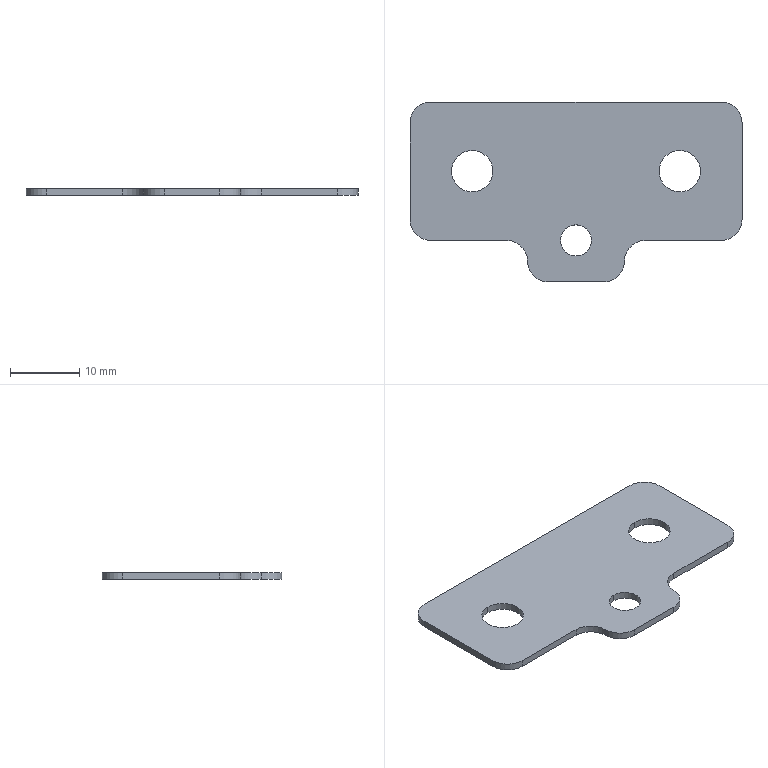Part | STEP file | J454-EBZ05-37-04-Part-1-1 | 1 solid | 22 faces | box 48 x 26 x 1 mm | volume 963.821 mm3 | cylinder 14 | plane 8 | commonest cylinder face diameters 6 x12 4.5 x2
STEP:
#1=CARTESIAN_POINT('',(24.,1.75,1.));
#2=VERTEX_POINT('',#1);
#3=CARTESIAN_POINT('',(24.,6.25,1.));
#4=VERTEX_POINT('',#3);
#5=CARTESIAN_POINT('',(24.,4.,1.));
#6=DIRECTION('',(0.,0.,-1.));
#7=DIRECTION('',(0.,1.,0.));
#8=AXIS2_PLACEMENT_3D('',#5,#6,#7);
#9=CIRCLE('',#8,2.25);
#10=EDGE_CURVE('',#2,#4,#9,.T.);
#11=ORIENTED_EDGE('',*,*,#10,.F.);
#12=CARTESIAN_POINT('',(24.,1.75,0.));
#13=VERTEX_POINT('',#12);
#14=CARTESIAN_POINT('',(24.,1.75,1.));
#15=DIRECTION('',(0.,0.,-1.));
#16=VECTOR('',#15,1000.);
#17=LINE('',#14,#16);
#18=EDGE_CURVE('',#2,#13,#17,.T.);
#19=ORIENTED_EDGE('',*,*,#18,.T.);
#20=CARTESIAN_POINT('',(24.,6.25,0.));
#21=VERTEX_POINT('',#20);
#22=CARTESIAN_POINT('',(24.,4.,0.));
#23=DIRECTION('',(0.,0.,1.));
#24=DIRECTION('',(0.,-1.,0.));
#25=AXIS2_PLACEMENT_3D('',#22,#23,#24);
#26=CIRCLE('',#25,2.25);
#27=EDGE_CURVE('',#21,#13,#26,.T.);
#28=ORIENTED_EDGE('',*,*,#27,.F.);
#29=CARTESIAN_POINT('',(24.,6.25,1.));
#30=DIRECTION('',(0.,0.,-1.));
#31=VECTOR('',#30,1000.);
#32=LINE('',#29,#31);
#33=EDGE_CURVE('',#4,#21,#32,.T.);
#34=ORIENTED_EDGE('',*,*,#33,.F.);
#35=EDGE_LOOP('',(#11,#19,#28,#34));
#36=FACE_OUTER_BOUND('',#35,.T.);
#37=CARTESIAN_POINT('',(24.,4.,1.));
#38=DIRECTION('',(0.,0.,-1.));
#39=DIRECTION('',(0.,1.,0.));
#40=AXIS2_PLACEMENT_3D('',#37,#38,#39);
#41=CYLINDRICAL_SURFACE('',#40,2.25);
#42=ADVANCED_FACE('',(#36),#41,.F.);
#43=CARTESIAN_POINT('',(9.,17.,0.));
#44=VERTEX_POINT('',#43);
#45=CARTESIAN_POINT('',(9.,11.,0.));
#46=VERTEX_POINT('',#45);
#47=CARTESIAN_POINT('',(9.,14.,0.));
#48=DIRECTION('',(0.,0.,1.));
#49=DIRECTION('',(0.,-1.,0.));
#50=AXIS2_PLACEMENT_3D('',#47,#48,#49);
#51=CIRCLE('',#50,3.);
#52=EDGE_CURVE('',#44,#46,#51,.T.);
#53=ORIENTED_EDGE('',*,*,#52,.F.);
#54=CARTESIAN_POINT('',(9.,17.,1.));
#55=VERTEX_POINT('',#54);
#56=CARTESIAN_POINT('',(9.,17.,0.));
#57=DIRECTION('',(0.,0.,1.));
#58=VECTOR('',#57,1000.);
#59=LINE('',#56,#58);
#60=EDGE_CURVE('',#44,#55,#59,.T.);
#61=ORIENTED_EDGE('',*,*,#60,.T.);
#62=CARTESIAN_POINT('',(9.,11.,1.));
#63=VERTEX_POINT('',#62);
#64=CARTESIAN_POINT('',(9.,14.,1.));
#65=DIRECTION('',(0.,0.,-1.));
#66=DIRECTION('',(0.,1.,0.));
#67=AXIS2_PLACEMENT_3D('',#64,#65,#66);
#68=CIRCLE('',#67,3.);
#69=EDGE_CURVE('',#63,#55,#68,.T.);
#70=ORIENTED_EDGE('',*,*,#69,.F.);
#71=CARTESIAN_POINT('',(9.,11.,0.));
#72=DIRECTION('',(0.,0.,1.));
#73=VECTOR('',#72,1000.);
#74=LINE('',#71,#73);
#75=EDGE_CURVE('',#46,#63,#74,.T.);
#76=ORIENTED_EDGE('',*,*,#75,.F.);
#77=EDGE_LOOP('',(#53,#61,#70,#76));
#78=FACE_OUTER_BOUND('',#77,.T.);
#79=CARTESIAN_POINT('',(9.,14.,0.));
#80=DIRECTION('',(0.,0.,1.));
#81=DIRECTION('',(0.,-1.,0.));
#82=AXIS2_PLACEMENT_3D('',#79,#80,#81);
#83=CYLINDRICAL_SURFACE('',#82,3.);
#84=ADVANCED_FACE('',(#78),#83,.F.);
#85=CARTESIAN_POINT('',(39.,17.,0.));
#86=VERTEX_POINT('',#85);
#87=CARTESIAN_POINT('',(39.,11.,0.));
#88=VERTEX_POINT('',#87);
#89=CARTESIAN_POINT('',(39.,14.,0.));
#90=DIRECTION('',(0.,0.,1.));
#91=DIRECTION('',(0.,-1.,0.));
#92=AXIS2_PLACEMENT_3D('',#89,#90,#91);
#93=CIRCLE('',#92,3.);
#94=EDGE_CURVE('',#86,#88,#93,.T.);
#95=ORIENTED_EDGE('',*,*,#94,.F.);
#96=CARTESIAN_POINT('',(39.,17.,1.));
#97=VERTEX_POINT('',#96);
#98=CARTESIAN_POINT('',(39.,17.,0.));
#99=DIRECTION('',(0.,0.,1.));
#100=VECTOR('',#99,1000.);
#101=LINE('',#98,#100);
#102=EDGE_CURVE('',#86,#97,#101,.T.);
#103=ORIENTED_EDGE('',*,*,#102,.T.);
#104=CARTESIAN_POINT('',(39.,11.,1.));
#105=VERTEX_POINT('',#104);
#106=CARTESIAN_POINT('',(39.,14.,1.));
#107=DIRECTION('',(0.,0.,-1.));
#108=DIRECTION('',(0.,1.,0.));
#109=AXIS2_PLACEMENT_3D('',#106,#107,#108);
#110=CIRCLE('',#109,3.);
#111=EDGE_CURVE('',#105,#97,#110,.T.);
#112=ORIENTED_EDGE('',*,*,#111,.F.);
#113=CARTESIAN_POINT('',(39.,11.,0.));
#114=DIRECTION('',(0.,0.,1.));
#115=VECTOR('',#114,1000.);
#116=LINE('',#113,#115);
#117=EDGE_CURVE('',#88,#105,#116,.T.);
#118=ORIENTED_EDGE('',*,*,#117,.F.);
#119=EDGE_LOOP('',(#95,#103,#112,#118));
#120=FACE_OUTER_BOUND('',#119,.T.);
#121=CARTESIAN_POINT('',(39.,14.,0.));
#122=DIRECTION('',(0.,0.,1.));
#123=DIRECTION('',(0.,-1.,0.));
#124=AXIS2_PLACEMENT_3D('',#121,#122,#123);
#125=CYLINDRICAL_SURFACE('',#124,3.);
#126=ADVANCED_FACE('',(#120),#125,.F.);
#127=CARTESIAN_POINT('',(14.,4.,0.));
#128=VERTEX_POINT('',#127);
#129=CARTESIAN_POINT('',(3.,4.,0.));
#130=VERTEX_POINT('',#129);
#131=CARTESIAN_POINT('',(24.,4.,0.));
#132=DIRECTION('',(-1.,0.,0.));
#133=VECTOR('',#132,1000.);
#134=LINE('',#131,#133);
#135=EDGE_CURVE('',#128,#130,#134,.T.);
#136=ORIENTED_EDGE('',*,*,#135,.F.);
#137=CARTESIAN_POINT('',(14.,4.,1.));
#138=VERTEX_POINT('',#137);
#139=CARTESIAN_POINT('',(14.,4.,1.));
#140=DIRECTION('',(0.,0.,1.));
#141=VECTOR('',#140,1000.);
#142=LINE('',#139,#141);
#143=EDGE_CURVE('',#128,#138,#142,.T.);
#144=ORIENTED_EDGE('',*,*,#143,.T.);
#145=CARTESIAN_POINT('',(3.,4.,1.));
#146=VERTEX_POINT('',#145);
#147=CARTESIAN_POINT('',(24.,4.,1.));
#148=DIRECTION('',(1.,0.,0.));
#149=VECTOR('',#148,1000.);
#150=LINE('',#147,#149);
#151=EDGE_CURVE('',#146,#138,#150,.T.);
#152=ORIENTED_EDGE('',*,*,#151,.F.);
#153=CARTESIAN_POINT('',(3.,4.,0.5));
#154=DIRECTION('',(0.,0.,-1.));
#155=VECTOR('',#154,1000.);
#156=LINE('',#153,#155);
#157=EDGE_CURVE('',#146,#130,#156,.T.);
#158=ORIENTED_EDGE('',*,*,#157,.T.);
#159=EDGE_LOOP('',(#136,#144,#152,#158));
#160=FACE_OUTER_BOUND('',#159,.T.);
#161=CARTESIAN_POINT('',(24.,4.,0.5));
#162=DIRECTION('',(0.,-1.,0.));
#163=DIRECTION('',(0.,0.,-1.));
#164=AXIS2_PLACEMENT_3D('',#161,#162,#163);
#165=PLANE('',#164);
#166=ADVANCED_FACE('',(#160),#165,.T.);
#167=CARTESIAN_POINT('',(45.,24.,1.));
#168=VERTEX_POINT('',#167);
#169=CARTESIAN_POINT('',(3.,24.,1.));
#170=VERTEX_POINT('',#169);
#171=CARTESIAN_POINT('',(24.,24.,1.));
#172=DIRECTION('',(-1.,0.,0.));
#173=VECTOR('',#172,1000.);
#174=LINE('',#171,#173);
#175=EDGE_CURVE('',#168,#170,#174,.T.);
#176=ORIENTED_EDGE('',*,*,#175,.F.);
#177=CARTESIAN_POINT('',(45.,24.,0.));
#178=VERTEX_POINT('',#177);
#179=CARTESIAN_POINT('',(45.,24.,0.5));
#180=DIRECTION('',(0.,0.,-1.));
#181=VECTOR('',#180,1000.);
#182=LINE('',#179,#181);
#183=EDGE_CURVE('',#168,#178,#182,.T.);
#184=ORIENTED_EDGE('',*,*,#183,.T.);
#185=CARTESIAN_POINT('',(3.,24.,0.));
#186=VERTEX_POINT('',#185);
#187=CARTESIAN_POINT('',(24.,24.,0.));
#188=DIRECTION('',(1.,0.,0.));
#189=VECTOR('',#188,1000.);
#190=LINE('',#187,#189);
#191=EDGE_CURVE('',#186,#178,#190,.T.);
#192=ORIENTED_EDGE('',*,*,#191,.F.);
#193=CARTESIAN_POINT('',(3.,24.,0.5));
#194=DIRECTION('',(0.,0.,1.));
#195=VECTOR('',#194,1000.);
#196=LINE('',#193,#195);
#197=EDGE_CURVE('',#186,#170,#196,.T.);
#198=ORIENTED_EDGE('',*,*,#197,.T.);
#199=EDGE_LOOP('',(#176,#184,#192,#198));
#200=FACE_OUTER_BOUND('',#199,.T.);
#201=CARTESIAN_POINT('',(24.,24.,0.5));
#202=DIRECTION('',(0.,1.,0.));
#203=DIRECTION('',(0.,0.,1.));
#204=AXIS2_PLACEMENT_3D('',#201,#202,#203);
#205=PLANE('',#204);
#206=ADVANCED_FACE('',(#200),#205,.T.);
#207=CARTESIAN_POINT('',(0.,7.,0.));
#208=VERTEX_POINT('',#207);
#209=CARTESIAN_POINT('',(0.,21.,0.));
#210=VERTEX_POINT('',#209);
#211=CARTESIAN_POINT('',(0.,4.,0.));
#212=DIRECTION('',(0.,1.,0.));
#213=VECTOR('',#212,1000.);
#214=LINE('',#211,#213);
#215=EDGE_CURVE('',#208,#210,#214,.T.);
#216=ORIENTED_EDGE('',*,*,#215,.F.);
#217=CARTESIAN_POINT('',(0.,7.,1.));
#218=VERTEX_POINT('',#217);
#219=CARTESIAN_POINT('',(0.,7.,0.5));
#220=DIRECTION('',(0.,0.,1.));
#221=VECTOR('',#220,1000.);
#222=LINE('',#219,#221);
#223=EDGE_CURVE('',#208,#218,#222,.T.);
#224=ORIENTED_EDGE('',*,*,#223,.T.);
#225=CARTESIAN_POINT('',(0.,21.,1.));
#226=VERTEX_POINT('',#225);
#227=CARTESIAN_POINT('',(0.,4.,1.));
#228=DIRECTION('',(0.,1.,0.));
#229=VECTOR('',#228,1000.);
#230=LINE('',#227,#229);
#231=EDGE_CURVE('',#218,#226,#230,.T.);
#232=ORIENTED_EDGE('',*,*,#231,.T.);
#233=CARTESIAN_POINT('',(0.,21.,0.5));
#234=DIRECTION('',(0.,0.,-1.));
#235=VECTOR('',#234,1000.);
#236=LINE('',#233,#235);
#237=EDGE_CURVE('',#226,#210,#236,.T.);
#238=ORIENTED_EDGE('',*,*,#237,.T.);
#239=EDGE_LOOP('',(#216,#224,#232,#238));
#240=FACE_OUTER_BOUND('',#239,.T.);
#241=CARTESIAN_POINT('',(0.,4.,0.5));
#242=DIRECTION('',(-1.,0.,0.));
#243=DIRECTION('',(0.,-1.,0.));
#244=AXIS2_PLACEMENT_3D('',#241,#242,#243);
#245=PLANE('',#244);
#246=ADVANCED_FACE('',(#240),#245,.T.);
#247=ORIENTED_EDGE('',*,*,#27,.T.);
#248=CARTESIAN_POINT('',(24.,4.,0.));
#249=DIRECTION('',(0.,0.,1.));
#250=DIRECTION('',(0.,-1.,0.));
#251=AXIS2_PLACEMENT_3D('',#248,#249,#250);
#252=CIRCLE('',#251,2.25);
#253=EDGE_CURVE('',#13,#21,#252,.T.);
#254=ORIENTED_EDGE('',*,*,#253,.T.);
#255=EDGE_LOOP('',(#247,#254));
#256=FACE_BOUND('',#255,.T.);
#257=CARTESIAN_POINT('',(9.,14.,0.));
#258=DIRECTION('',(0.,0.,1.));
#259=DIRECTION('',(0.,-1.,0.));
#260=AXIS2_PLACEMENT_3D('',#257,#258,#259);
#261=CIRCLE('',#260,3.);
#262=EDGE_CURVE('',#46,#44,#261,.T.);
#263=ORIENTED_EDGE('',*,*,#262,.T.);
#264=ORIENTED_EDGE('',*,*,#52,.T.);
#265=EDGE_LOOP('',(#263,#264));
#266=FACE_BOUND('',#265,.T.);
#267=CARTESIAN_POINT('',(39.,14.,0.));
#268=DIRECTION('',(0.,0.,1.));
#269=DIRECTION('',(0.,-1.,0.));
#270=AXIS2_PLACEMENT_3D('',#267,#268,#269);
#271=CIRCLE('',#270,3.);
#272=EDGE_CURVE('',#88,#86,#271,.T.);
#273=ORIENTED_EDGE('',*,*,#272,.T.);
#274=ORIENTED_EDGE('',*,*,#94,.T.);
#275=EDGE_LOOP('',(#273,#274));
#276=FACE_BOUND('',#275,.T.);
#277=CARTESIAN_POINT('',(28.,-2.,0.));
#278=VERTEX_POINT('',#277);
#279=CARTESIAN_POINT('',(20.,-2.,0.));
#280=VERTEX_POINT('',#279);
#281=CARTESIAN_POINT('',(24.,-2.,0.));
#282=DIRECTION('',(-1.,0.,0.));
#283=VECTOR('',#282,1000.);
#284=LINE('',#281,#283);
#285=EDGE_CURVE('',#278,#280,#284,.T.);
#286=ORIENTED_EDGE('',*,*,#285,.T.);
#287=CARTESIAN_POINT('',(17.,1.,0.));
#288=VERTEX_POINT('',#287);
#289=CARTESIAN_POINT('',(20.,1.,0.));
#290=DIRECTION('',(0.,0.,-1.));
#291=DIRECTION('',(0.,1.,0.));
#292=AXIS2_PLACEMENT_3D('',#289,#290,#291);
#293=CIRCLE('',#292,3.);
#294=EDGE_CURVE('',#280,#288,#293,.T.);
#295=ORIENTED_EDGE('',*,*,#294,.T.);
#296=CARTESIAN_POINT('',(14.,1.,0.));
#297=DIRECTION('',(0.,0.,1.));
#298=DIRECTION('',(0.,1.,0.));
#299=AXIS2_PLACEMENT_3D('',#296,#297,#298);
#300=CIRCLE('',#299,3.);
#301=EDGE_CURVE('',#288,#128,#300,.T.);
#302=ORIENTED_EDGE('',*,*,#301,.T.);
#303=ORIENTED_EDGE('',*,*,#135,.T.);
#304=CARTESIAN_POINT('',(3.,7.,0.));
#305=DIRECTION('',(0.,0.,-1.));
#306=DIRECTION('',(0.,1.,0.));
#307=AXIS2_PLACEMENT_3D('',#304,#305,#306);
#308=CIRCLE('',#307,3.);
#309=EDGE_CURVE('',#130,#208,#308,.T.);
#310=ORIENTED_EDGE('',*,*,#309,.T.);
#311=ORIENTED_EDGE('',*,*,#215,.T.);
#312=CARTESIAN_POINT('',(3.,21.,0.));
#313=DIRECTION('',(0.,0.,-1.));
#314=DIRECTION('',(0.,1.,0.));
#315=AXIS2_PLACEMENT_3D('',#312,#313,#314);
#316=CIRCLE('',#315,3.);
#317=EDGE_CURVE('',#210,#186,#316,.T.);
#318=ORIENTED_EDGE('',*,*,#317,.T.);
#319=ORIENTED_EDGE('',*,*,#191,.T.);
#320=CARTESIAN_POINT('',(48.,21.,0.));
#321=VERTEX_POINT('',#320);
#322=CARTESIAN_POINT('',(45.,21.,0.));
#323=DIRECTION('',(0.,0.,-1.));
#324=DIRECTION('',(0.,1.,0.));
#325=AXIS2_PLACEMENT_3D('',#322,#323,#324);
#326=CIRCLE('',#325,3.);
#327=EDGE_CURVE('',#178,#321,#326,.T.);
#328=ORIENTED_EDGE('',*,*,#327,.T.);
#329=CARTESIAN_POINT('',(48.,7.,0.));
#330=VERTEX_POINT('',#329);
#331=CARTESIAN_POINT('',(48.,4.,0.));
#332=DIRECTION('',(0.,1.,0.));
#333=VECTOR('',#332,1000.);
#334=LINE('',#331,#333);
#335=EDGE_CURVE('',#330,#321,#334,.T.);
#336=ORIENTED_EDGE('',*,*,#335,.F.);
#337=CARTESIAN_POINT('',(45.,4.,0.));
#338=VERTEX_POINT('',#337);
#339=CARTESIAN_POINT('',(45.,7.,0.));
#340=DIRECTION('',(0.,0.,-1.));
#341=DIRECTION('',(0.,1.,0.));
#342=AXIS2_PLACEMENT_3D('',#339,#340,#341);
#343=CIRCLE('',#342,3.);
#344=EDGE_CURVE('',#330,#338,#343,.T.);
#345=ORIENTED_EDGE('',*,*,#344,.T.);
#346=CARTESIAN_POINT('',(34.,4.,0.));
#347=VERTEX_POINT('',#346);
#348=CARTESIAN_POINT('',(24.,4.,0.));
#349=DIRECTION('',(-1.,0.,0.));
#350=VECTOR('',#349,1000.);
#351=LINE('',#348,#350);
#352=EDGE_CURVE('',#338,#347,#351,.T.);
#353=ORIENTED_EDGE('',*,*,#352,.T.);
#354=CARTESIAN_POINT('',(31.,1.,0.));
#355=VERTEX_POINT('',#354);
#356=CARTESIAN_POINT('',(34.,1.,0.));
#357=DIRECTION('',(0.,0.,1.));
#358=DIRECTION('',(0.,1.,0.));
#359=AXIS2_PLACEMENT_3D('',#356,#357,#358);
#360=CIRCLE('',#359,3.);
#361=EDGE_CURVE('',#347,#355,#360,.T.);
#362=ORIENTED_EDGE('',*,*,#361,.T.);
#363=CARTESIAN_POINT('',(28.,1.,0.));
#364=DIRECTION('',(0.,0.,-1.));
#365=DIRECTION('',(0.,1.,0.));
#366=AXIS2_PLACEMENT_3D('',#363,#364,#365);
#367=CIRCLE('',#366,3.);
#368=EDGE_CURVE('',#355,#278,#367,.T.);
#369=ORIENTED_EDGE('',*,*,#368,.T.);
#370=EDGE_LOOP('',(#286,#295,#302,#303,#310,#311,#318,#319,#328,#336,#345,#353,#362,#369));
#371=FACE_OUTER_BOUND('',#370,.T.);
#372=CARTESIAN_POINT('',(24.,4.,0.));
#373=DIRECTION('',(0.,0.,-1.));
#374=DIRECTION('',(0.,1.,0.));
#375=AXIS2_PLACEMENT_3D('',#372,#373,#374);
#376=PLANE('',#375);
#377=ADVANCED_FACE('',(#256,#266,#276,#371),#376,.T.);
#378=CARTESIAN_POINT('',(48.,7.,1.));
#379=VERTEX_POINT('',#378);
#380=CARTESIAN_POINT('',(48.,21.,1.));
#381=VERTEX_POINT('',#380);
#382=CARTESIAN_POINT('',(48.,4.,1.));
#383=DIRECTION('',(0.,1.,0.));
#384=VECTOR('',#383,1000.);
#385=LINE('',#382,#384);
#386=EDGE_CURVE('',#379,#381,#385,.T.);
#387=ORIENTED_EDGE('',*,*,#386,.F.);
#388=CARTESIAN_POINT('',(48.,7.,0.5));
#389=DIRECTION('',(0.,0.,-1.));
#390=VECTOR('',#389,1000.);
#391=LINE('',#388,#390);
#392=EDGE_CURVE('',#379,#330,#391,.T.);
#393=ORIENTED_EDGE('',*,*,#392,.T.);
#394=ORIENTED_EDGE('',*,*,#335,.T.);
#395=CARTESIAN_POINT('',(48.,21.,0.5));
#396=DIRECTION('',(0.,0.,1.));
#397=VECTOR('',#396,1000.);
#398=LINE('',#395,#397);
#399=EDGE_CURVE('',#321,#381,#398,.T.);
#400=ORIENTED_EDGE('',*,*,#399,.T.);
#401=EDGE_LOOP('',(#387,#393,#394,#400));
#402=FACE_OUTER_BOUND('',#401,.T.);
#403=CARTESIAN_POINT('',(48.,4.,0.5));
#404=DIRECTION('',(1.,0.,0.));
#405=DIRECTION('',(0.,1.,0.));
#406=AXIS2_PLACEMENT_3D('',#403,#404,#405);
#407=PLANE('',#406);
#408=ADVANCED_FACE('',(#402),#407,.T.);
#409=CARTESIAN_POINT('',(34.,4.,1.));
#410=VERTEX_POINT('',#409);
#411=CARTESIAN_POINT('',(45.,4.,1.));
#412=VERTEX_POINT('',#411);
#413=CARTESIAN_POINT('',(24.,4.,1.));
#414=DIRECTION('',(1.,0.,0.));
#415=VECTOR('',#414,1000.);
#416=LINE('',#413,#415);
#417=EDGE_CURVE('',#410,#412,#416,.T.);
#418=ORIENTED_EDGE('',*,*,#417,.F.);
#419=CARTESIAN_POINT('',(34.,4.,0.));
#420=DIRECTION('',(0.,0.,-1.));
#421=VECTOR('',#420,1000.);
#422=LINE('',#419,#421);
#423=EDGE_CURVE('',#410,#347,#422,.T.);
#424=ORIENTED_EDGE('',*,*,#423,.T.);
#425=ORIENTED_EDGE('',*,*,#352,.F.);
#426=CARTESIAN_POINT('',(45.,4.,0.5));
#427=DIRECTION('',(0.,0.,1.));
#428=VECTOR('',#427,1000.);
#429=LINE('',#426,#428);
#430=EDGE_CURVE('',#338,#412,#429,.T.);
#431=ORIENTED_EDGE('',*,*,#430,.T.);
#432=EDGE_LOOP('',(#418,#424,#425,#431));
#433=FACE_OUTER_BOUND('',#432,.T.);
#434=CARTESIAN_POINT('',(24.,4.,0.5));
#435=DIRECTION('',(0.,-1.,0.));
#436=DIRECTION('',(0.,0.,-1.));
#437=AXIS2_PLACEMENT_3D('',#434,#435,#436);
#438=PLANE('',#437);
#439=ADVANCED_FACE('',(#433),#438,.T.);
#440=CARTESIAN_POINT('',(24.,4.,1.));
#441=DIRECTION('',(0.,0.,-1.));
#442=DIRECTION('',(0.,1.,0.));
#443=AXIS2_PLACEMENT_3D('',#440,#441,#442);
#444=CIRCLE('',#443,2.25);
#445=EDGE_CURVE('',#4,#2,#444,.T.);
#446=ORIENTED_EDGE('',*,*,#445,.T.);
#447=ORIENTED_EDGE('',*,*,#10,.T.);
#448=EDGE_LOOP('',(#446,#447));
#449=FACE_BOUND('',#448,.T.);
#450=ORIENTED_EDGE('',*,*,#69,.T.);
#451=CARTESIAN_POINT('',(9.,14.,1.));
#452=DIRECTION('',(0.,0.,-1.));
#453=DIRECTION('',(0.,1.,0.));
#454=AXIS2_PLACEMENT_3D('',#451,#452,#453);
#455=CIRCLE('',#454,3.);
#456=EDGE_CURVE('',#55,#63,#455,.T.);
#457=ORIENTED_EDGE('',*,*,#456,.T.);
#458=EDGE_LOOP('',(#450,#457));
#459=FACE_BOUND('',#458,.T.);
#460=ORIENTED_EDGE('',*,*,#111,.T.);
#461=CARTESIAN_POINT('',(39.,14.,1.));
#462=DIRECTION('',(0.,0.,-1.));
#463=DIRECTION('',(0.,1.,0.));
#464=AXIS2_PLACEMENT_3D('',#461,#462,#463);
#465=CIRCLE('',#464,3.);
#466=EDGE_CURVE('',#97,#105,#465,.T.);
#467=ORIENTED_EDGE('',*,*,#466,.T.);
#468=EDGE_LOOP('',(#460,#467));
#469=FACE_BOUND('',#468,.T.);
#470=ORIENTED_EDGE('',*,*,#151,.T.);
#471=CARTESIAN_POINT('',(17.,1.,1.));
#472=VERTEX_POINT('',#471);
#473=CARTESIAN_POINT('',(14.,1.,1.));
#474=DIRECTION('',(0.,0.,-1.));
#475=DIRECTION('',(0.,-1.,0.));
#476=AXIS2_PLACEMENT_3D('',#473,#474,#475);
#477=CIRCLE('',#476,3.);
#478=EDGE_CURVE('',#138,#472,#477,.T.);
#479=ORIENTED_EDGE('',*,*,#478,.T.);
#480=CARTESIAN_POINT('',(20.,-2.,1.));
#481=VERTEX_POINT('',#480);
#482=CARTESIAN_POINT('',(20.,1.,1.));
#483=DIRECTION('',(0.,0.,1.));
#484=DIRECTION('',(0.,-1.,0.));
#485=AXIS2_PLACEMENT_3D('',#482,#483,#484);
#486=CIRCLE('',#485,3.);
#487=EDGE_CURVE('',#472,#481,#486,.T.);
#488=ORIENTED_EDGE('',*,*,#487,.T.);
#489=CARTESIAN_POINT('',(28.,-2.,1.));
#490=VERTEX_POINT('',#489);
#491=CARTESIAN_POINT('',(24.,-2.,1.));
#492=DIRECTION('',(1.,0.,0.));
#493=VECTOR('',#492,1000.);
#494=LINE('',#491,#493);
#495=EDGE_CURVE('',#481,#490,#494,.T.);
#496=ORIENTED_EDGE('',*,*,#495,.T.);
#497=CARTESIAN_POINT('',(31.,1.,1.));
#498=VERTEX_POINT('',#497);
#499=CARTESIAN_POINT('',(28.,1.,1.));
#500=DIRECTION('',(0.,0.,1.));
#501=DIRECTION('',(0.,-1.,0.));
#502=AXIS2_PLACEMENT_3D('',#499,#500,#501);
#503=CIRCLE('',#502,3.);
#504=EDGE_CURVE('',#490,#498,#503,.T.);
#505=ORIENTED_EDGE('',*,*,#504,.T.);
#506=CARTESIAN_POINT('',(34.,1.,1.));
#507=DIRECTION('',(0.,0.,-1.));
#508=DIRECTION('',(0.,-1.,0.));
#509=AXIS2_PLACEMENT_3D('',#506,#507,#508);
#510=CIRCLE('',#509,3.);
#511=EDGE_CURVE('',#498,#410,#510,.T.);
#512=ORIENTED_EDGE('',*,*,#511,.T.);
#513=ORIENTED_EDGE('',*,*,#417,.T.);
#514=CARTESIAN_POINT('',(45.,7.,1.));
#515=DIRECTION('',(0.,0.,1.));
#516=DIRECTION('',(0.,-1.,0.));
#517=AXIS2_PLACEMENT_3D('',#514,#515,#516);
#518=CIRCLE('',#517,3.);
#519=EDGE_CURVE('',#412,#379,#518,.T.);
#520=ORIENTED_EDGE('',*,*,#519,.T.);
#521=ORIENTED_EDGE('',*,*,#386,.T.);
#522=CARTESIAN_POINT('',(45.,21.,1.));
#523=DIRECTION('',(0.,0.,1.));
#524=DIRECTION('',(0.,-1.,0.));
#525=AXIS2_PLACEMENT_3D('',#522,#523,#524);
#526=CIRCLE('',#525,3.);
#527=EDGE_CURVE('',#381,#168,#526,.T.);
#528=ORIENTED_EDGE('',*,*,#527,.T.);
#529=ORIENTED_EDGE('',*,*,#175,.T.);
#530=CARTESIAN_POINT('',(3.,21.,1.));
#531=DIRECTION('',(0.,0.,1.));
#532=DIRECTION('',(0.,-1.,0.));
#533=AXIS2_PLACEMENT_3D('',#530,#531,#532);
#534=CIRCLE('',#533,3.);
#535=EDGE_CURVE('',#170,#226,#534,.T.);
#536=ORIENTED_EDGE('',*,*,#535,.T.);
#537=ORIENTED_EDGE('',*,*,#231,.F.);
#538=CARTESIAN_POINT('',(3.,7.,1.));
#539=DIRECTION('',(0.,0.,1.));
#540=DIRECTION('',(0.,-1.,0.));
#541=AXIS2_PLACEMENT_3D('',#538,#539,#540);
#542=CIRCLE('',#541,3.);
#543=EDGE_CURVE('',#218,#146,#542,.T.);
#544=ORIENTED_EDGE('',*,*,#543,.T.);
#545=EDGE_LOOP('',(#470,#479,#488,#496,#505,#512,#513,#520,#521,#528,#529,#536,#537,#544));
#546=FACE_OUTER_BOUND('',#545,.T.);
#547=CARTESIAN_POINT('',(24.,4.,1.));
#548=DIRECTION('',(0.,0.,1.));
#549=DIRECTION('',(0.,-1.,0.));
#550=AXIS2_PLACEMENT_3D('',#547,#548,#549);
#551=PLANE('',#550);
#552=ADVANCED_FACE('',(#449,#459,#469,#546),#551,.T.);
#553=ORIENTED_EDGE('',*,*,#327,.F.);
#554=ORIENTED_EDGE('',*,*,#183,.F.);
#555=ORIENTED_EDGE('',*,*,#527,.F.);
#556=ORIENTED_EDGE('',*,*,#399,.F.);
#557=EDGE_LOOP('',(#553,#554,#555,#556));
#558=FACE_OUTER_BOUND('',#557,.T.);
#559=CARTESIAN_POINT('',(45.,21.,0.5));
#560=DIRECTION('',(0.,0.,1.));
#561=DIRECTION('',(0.,-1.,0.));
#562=AXIS2_PLACEMENT_3D('',#559,#560,#561);
#563=CYLINDRICAL_SURFACE('',#562,3.);
#564=ADVANCED_FACE('',(#558),#563,.T.);
#565=ORIENTED_EDGE('',*,*,#535,.F.);
#566=ORIENTED_EDGE('',*,*,#197,.F.);
#567=ORIENTED_EDGE('',*,*,#317,.F.);
#568=ORIENTED_EDGE('',*,*,#237,.F.);
#569=EDGE_LOOP('',(#565,#566,#567,#568));
#570=FACE_OUTER_BOUND('',#569,.T.);
#571=CARTESIAN_POINT('',(3.,21.,0.5));
#572=DIRECTION('',(0.,0.,-1.));
#573=DIRECTION('',(0.,1.,0.));
#574=AXIS2_PLACEMENT_3D('',#571,#572,#573);
#575=CYLINDRICAL_SURFACE('',#574,3.);
#576=ADVANCED_FACE('',(#570),#575,.T.);
#577=ORIENTED_EDGE('',*,*,#102,.F.);
#578=ORIENTED_EDGE('',*,*,#272,.F.);
#579=ORIENTED_EDGE('',*,*,#117,.T.);
#580=ORIENTED_EDGE('',*,*,#466,.F.);
#581=EDGE_LOOP('',(#577,#578,#579,#580));
#582=FACE_OUTER_BOUND('',#581,.T.);
#583=CARTESIAN_POINT('',(39.,14.,0.));
#584=DIRECTION('',(0.,0.,1.));
#585=DIRECTION('',(0.,-1.,0.));
#586=AXIS2_PLACEMENT_3D('',#583,#584,#585);
#587=CYLINDRICAL_SURFACE('',#586,3.);
#588=ADVANCED_FACE('',(#582),#587,.F.);
#589=ORIENTED_EDGE('',*,*,#60,.F.);
#590=ORIENTED_EDGE('',*,*,#262,.F.);
#591=ORIENTED_EDGE('',*,*,#75,.T.);
#592=ORIENTED_EDGE('',*,*,#456,.F.);
#593=EDGE_LOOP('',(#589,#590,#591,#592));
#594=FACE_OUTER_BOUND('',#593,.T.);
#595=CARTESIAN_POINT('',(9.,14.,0.));
#596=DIRECTION('',(0.,0.,1.));
#597=DIRECTION('',(0.,-1.,0.));
#598=AXIS2_PLACEMENT_3D('',#595,#596,#597);
#599=CYLINDRICAL_SURFACE('',#598,3.);
#600=ADVANCED_FACE('',(#594),#599,.F.);
#601=ORIENTED_EDGE('',*,*,#495,.F.);
#602=CARTESIAN_POINT('',(20.,-2.,0.5));
#603=DIRECTION('',(0.,0.,-1.));
#604=VECTOR('',#603,1000.);
#605=LINE('',#602,#604);
#606=EDGE_CURVE('',#481,#280,#605,.T.);
#607=ORIENTED_EDGE('',*,*,#606,.T.);
#608=ORIENTED_EDGE('',*,*,#285,.F.);
#609=CARTESIAN_POINT('',(28.,-2.,0.5));
#610=DIRECTION('',(0.,0.,1.));
#611=VECTOR('',#610,1000.);
#612=LINE('',#609,#611);
#613=EDGE_CURVE('',#278,#490,#612,.T.);
#614=ORIENTED_EDGE('',*,*,#613,.T.);
#615=EDGE_LOOP('',(#601,#607,#608,#614));
#616=FACE_OUTER_BOUND('',#615,.T.);
#617=CARTESIAN_POINT('',(24.,-2.,0.5));
#618=DIRECTION('',(0.,-1.,0.));
#619=DIRECTION('',(0.,0.,-1.));
#620=AXIS2_PLACEMENT_3D('',#617,#618,#619);
#621=PLANE('',#620);
#622=ADVANCED_FACE('',(#616),#621,.T.);
#623=ORIENTED_EDGE('',*,*,#309,.F.);
#624=ORIENTED_EDGE('',*,*,#157,.F.);
#625=ORIENTED_EDGE('',*,*,#543,.F.);
#626=ORIENTED_EDGE('',*,*,#223,.F.);
#627=EDGE_LOOP('',(#623,#624,#625,#626));
#628=FACE_OUTER_BOUND('',#627,.T.);
#629=CARTESIAN_POINT('',(3.,7.,0.5));
#630=DIRECTION('',(0.,0.,1.));
#631=DIRECTION('',(0.,-1.,0.));
#632=AXIS2_PLACEMENT_3D('',#629,#630,#631);
#633=CYLINDRICAL_SURFACE('',#632,3.);
#634=ADVANCED_FACE('',(#628),#633,.T.);
#635=ORIENTED_EDGE('',*,*,#519,.F.);
#636=ORIENTED_EDGE('',*,*,#430,.F.);
#637=ORIENTED_EDGE('',*,*,#344,.F.);
#638=ORIENTED_EDGE('',*,*,#392,.F.);
#639=EDGE_LOOP('',(#635,#636,#637,#638));
#640=FACE_OUTER_BOUND('',#639,.T.);
#641=CARTESIAN_POINT('',(45.,7.,0.5));
#642=DIRECTION('',(0.,0.,-1.));
#643=DIRECTION('',(0.,1.,0.));
#644=AXIS2_PLACEMENT_3D('',#641,#642,#643);
#645=CYLINDRICAL_SURFACE('',#644,3.);
#646=ADVANCED_FACE('',(#640),#645,.T.);
#647=ORIENTED_EDGE('',*,*,#606,.F.);
#648=ORIENTED_EDGE('',*,*,#487,.F.);
#649=CARTESIAN_POINT('',(17.,1.,0.5));
#650=DIRECTION('',(0.,0.,1.));
#651=VECTOR('',#650,1000.);
#652=LINE('',#649,#651);
#653=EDGE_CURVE('',#288,#472,#652,.T.);
#654=ORIENTED_EDGE('',*,*,#653,.F.);
#655=ORIENTED_EDGE('',*,*,#294,.F.);
#656=EDGE_LOOP('',(#647,#648,#654,#655));
#657=FACE_OUTER_BOUND('',#656,.T.);
#658=CARTESIAN_POINT('',(20.,1.,0.5));
#659=DIRECTION('',(0.,0.,1.));
#660=DIRECTION('',(0.,-1.,0.));
#661=AXIS2_PLACEMENT_3D('',#658,#659,#660);
#662=CYLINDRICAL_SURFACE('',#661,3.);
#663=ADVANCED_FACE('',(#657),#662,.T.);
#664=ORIENTED_EDGE('',*,*,#478,.F.);
#665=ORIENTED_EDGE('',*,*,#143,.F.);
#666=ORIENTED_EDGE('',*,*,#301,.F.);
#667=ORIENTED_EDGE('',*,*,#653,.T.);
#668=EDGE_LOOP('',(#664,#665,#666,#667));
#669=FACE_OUTER_BOUND('',#668,.T.);
#670=CARTESIAN_POINT('',(14.,1.,0.5));
#671=DIRECTION('',(0.,0.,1.));
#672=DIRECTION('',(0.,-1.,0.));
#673=AXIS2_PLACEMENT_3D('',#670,#671,#672);
#674=CYLINDRICAL_SURFACE('',#673,3.);
#675=ADVANCED_FACE('',(#669),#674,.F.);
#676=ORIENTED_EDGE('',*,*,#423,.F.);
#677=ORIENTED_EDGE('',*,*,#511,.F.);
#678=CARTESIAN_POINT('',(31.,1.,1.));
#679=DIRECTION('',(0.,0.,1.));
#680=VECTOR('',#679,1000.);
#681=LINE('',#678,#680);
#682=EDGE_CURVE('',#355,#498,#681,.T.);
#683=ORIENTED_EDGE('',*,*,#682,.F.);
#684=ORIENTED_EDGE('',*,*,#361,.F.);
#685=EDGE_LOOP('',(#676,#677,#683,#684));
#686=FACE_OUTER_BOUND('',#685,.T.);
#687=CARTESIAN_POINT('',(34.,1.,0.5));
#688=DIRECTION('',(0.,0.,-1.));
#689=DIRECTION('',(0.,1.,0.));
#690=AXIS2_PLACEMENT_3D('',#687,#688,#689);
#691=CYLINDRICAL_SURFACE('',#690,3.);
#692=ADVANCED_FACE('',(#686),#691,.F.);
#693=ORIENTED_EDGE('',*,*,#504,.F.);
#694=ORIENTED_EDGE('',*,*,#613,.F.);
#695=ORIENTED_EDGE('',*,*,#368,.F.);
#696=ORIENTED_EDGE('',*,*,#682,.T.);
#697=EDGE_LOOP('',(#693,#694,#695,#696));
#698=FACE_OUTER_BOUND('',#697,.T.);
#699=CARTESIAN_POINT('',(28.,1.,0.5));
#700=DIRECTION('',(0.,0.,-1.));
#701=DIRECTION('',(0.,1.,0.));
#702=AXIS2_PLACEMENT_3D('',#699,#700,#701);
#703=CYLINDRICAL_SURFACE('',#702,3.);
#704=ADVANCED_FACE('',(#698),#703,.T.);
#705=ORIENTED_EDGE('',*,*,#18,.F.);
#706=ORIENTED_EDGE('',*,*,#445,.F.);
#707=ORIENTED_EDGE('',*,*,#33,.T.);
#708=ORIENTED_EDGE('',*,*,#253,.F.);
#709=EDGE_LOOP('',(#705,#706,#707,#708));
#710=FACE_OUTER_BOUND('',#709,.T.);
#711=CARTESIAN_POINT('',(24.,4.,1.));
#712=DIRECTION('',(0.,0.,-1.));
#713=DIRECTION('',(0.,1.,0.));
#714=AXIS2_PLACEMENT_3D('',#711,#712,#713);
#715=CYLINDRICAL_SURFACE('',#714,2.25);
#716=ADVANCED_FACE('',(#710),#715,.F.);
#717=CLOSED_SHELL('',(#42,#84,#126,#166,#206,#246,#377,#408,#439,#552,#564,#576,#588,#600,#622,#634,#646,#663,#675,#692,#704,#716));
#718=MANIFOLD_SOLID_BREP('',#717);
#719=CARTESIAN_POINT('',(0.,0.,0.));
#720=DIRECTION('',(0.,0.,1.));
#721=DIRECTION('',(1.,0.,0.));
#722=AXIS2_PLACEMENT_3D('',#719,#720,#721);
#723=(LENGTH_UNIT()NAMED_UNIT(*)SI_UNIT(.MILLI.,.METRE.));
#724=UNCERTAINTY_MEASURE_WITH_UNIT(LENGTH_MEASURE(0.00001),#723,'','');
#725=(NAMED_UNIT(*)PLANE_ANGLE_UNIT()SI_UNIT($,.RADIAN.));
#726=(NAMED_UNIT(*)SI_UNIT($,.STERADIAN.)SOLID_ANGLE_UNIT());
#727=(GEOMETRIC_REPRESENTATION_CONTEXT(3)GLOBAL_UNCERTAINTY_ASSIGNED_CONTEXT((#724))GLOBAL_UNIT_ASSIGNED_CONTEXT((#723,#725,#726))REPRESENTATION_CONTEXT('',''));
#728=ADVANCED_BREP_SHAPE_REPRESENTATION('',(#718,#722),#727);